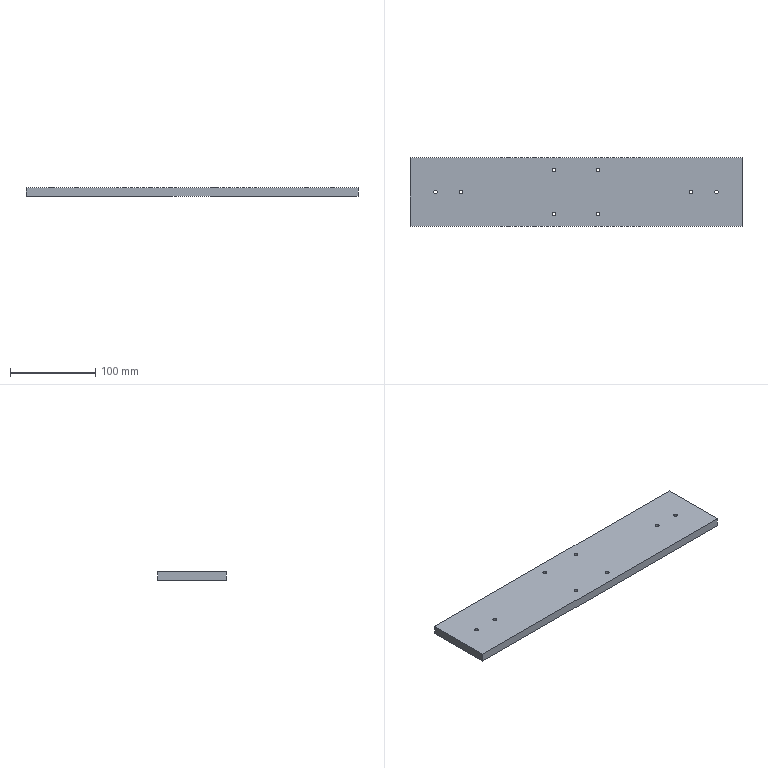Part | STEP file | X77-04402 | 1 solid | 22 faces | box 390 x 80 x 10 mm | volume 310892 mm3 | cylinder 16 | plane 6 | commonest cylinder face diameters 4.2 x16
STEP:
#1=CARTESIAN_POINT('',(162.9,0.,0.));
#2=VERTEX_POINT('',#1);
#3=CARTESIAN_POINT('',(167.1,0.,0.));
#4=VERTEX_POINT('',#3);
#5=CARTESIAN_POINT('',(165.,0.,0.));
#6=DIRECTION('',(0.,0.,1.));
#7=DIRECTION('',(1.,0.,0.));
#8=AXIS2_PLACEMENT_3D('',#5,#6,#7);
#9=CIRCLE('',#8,2.1);
#10=EDGE_CURVE('',#2,#4,#9,.T.);
#11=ORIENTED_EDGE('',*,*,#10,.F.);
#12=CARTESIAN_POINT('',(162.9,0.,10.));
#13=VERTEX_POINT('',#12);
#14=CARTESIAN_POINT('',(162.9,0.,10.));
#15=DIRECTION('',(0.,0.,1.));
#16=VECTOR('',#15,1000.);
#17=LINE('',#14,#16);
#18=EDGE_CURVE('',#2,#13,#17,.T.);
#19=ORIENTED_EDGE('',*,*,#18,.T.);
#20=CARTESIAN_POINT('',(167.1,0.,10.));
#21=VERTEX_POINT('',#20);
#22=CARTESIAN_POINT('',(165.,0.,10.));
#23=DIRECTION('',(0.,0.,1.));
#24=DIRECTION('',(1.,0.,0.));
#25=AXIS2_PLACEMENT_3D('',#22,#23,#24);
#26=CIRCLE('',#25,2.1);
#27=EDGE_CURVE('',#13,#21,#26,.T.);
#28=ORIENTED_EDGE('',*,*,#27,.T.);
#29=CARTESIAN_POINT('',(167.1,0.,10.));
#30=DIRECTION('',(0.,0.,1.));
#31=VECTOR('',#30,1000.);
#32=LINE('',#29,#31);
#33=EDGE_CURVE('',#4,#21,#32,.T.);
#34=ORIENTED_EDGE('',*,*,#33,.F.);
#35=EDGE_LOOP('',(#11,#19,#28,#34));
#36=FACE_OUTER_BOUND('',#35,.T.);
#37=CARTESIAN_POINT('',(165.,0.,10.));
#38=DIRECTION('',(0.,0.,1.));
#39=DIRECTION('',(1.,0.,0.));
#40=AXIS2_PLACEMENT_3D('',#37,#38,#39);
#41=CYLINDRICAL_SURFACE('',#40,2.1);
#42=ADVANCED_FACE('',(#36),#41,.F.);
#43=CARTESIAN_POINT('',(132.9,0.,0.));
#44=VERTEX_POINT('',#43);
#45=CARTESIAN_POINT('',(137.1,0.,0.));
#46=VERTEX_POINT('',#45);
#47=CARTESIAN_POINT('',(135.,0.,0.));
#48=DIRECTION('',(0.,0.,1.));
#49=DIRECTION('',(1.,0.,0.));
#50=AXIS2_PLACEMENT_3D('',#47,#48,#49);
#51=CIRCLE('',#50,2.1);
#52=EDGE_CURVE('',#44,#46,#51,.T.);
#53=ORIENTED_EDGE('',*,*,#52,.F.);
#54=CARTESIAN_POINT('',(132.9,0.,10.));
#55=VERTEX_POINT('',#54);
#56=CARTESIAN_POINT('',(132.9,0.,10.));
#57=DIRECTION('',(0.,0.,1.));
#58=VECTOR('',#57,1000.);
#59=LINE('',#56,#58);
#60=EDGE_CURVE('',#44,#55,#59,.T.);
#61=ORIENTED_EDGE('',*,*,#60,.T.);
#62=CARTESIAN_POINT('',(137.1,0.,10.));
#63=VERTEX_POINT('',#62);
#64=CARTESIAN_POINT('',(135.,0.,10.));
#65=DIRECTION('',(0.,0.,1.));
#66=DIRECTION('',(1.,0.,0.));
#67=AXIS2_PLACEMENT_3D('',#64,#65,#66);
#68=CIRCLE('',#67,2.1);
#69=EDGE_CURVE('',#55,#63,#68,.T.);
#70=ORIENTED_EDGE('',*,*,#69,.T.);
#71=CARTESIAN_POINT('',(137.1,0.,10.));
#72=DIRECTION('',(0.,0.,1.));
#73=VECTOR('',#72,1000.);
#74=LINE('',#71,#73);
#75=EDGE_CURVE('',#46,#63,#74,.T.);
#76=ORIENTED_EDGE('',*,*,#75,.F.);
#77=EDGE_LOOP('',(#53,#61,#70,#76));
#78=FACE_OUTER_BOUND('',#77,.T.);
#79=CARTESIAN_POINT('',(135.,0.,10.));
#80=DIRECTION('',(0.,0.,1.));
#81=DIRECTION('',(1.,0.,0.));
#82=AXIS2_PLACEMENT_3D('',#79,#80,#81);
#83=CYLINDRICAL_SURFACE('',#82,2.1);
#84=ADVANCED_FACE('',(#78),#83,.F.);
#85=CARTESIAN_POINT('',(-137.1,0.,0.));
#86=VERTEX_POINT('',#85);
#87=CARTESIAN_POINT('',(-132.9,0.,0.));
#88=VERTEX_POINT('',#87);
#89=CARTESIAN_POINT('',(-135.,0.,0.));
#90=DIRECTION('',(0.,0.,1.));
#91=DIRECTION('',(1.,0.,0.));
#92=AXIS2_PLACEMENT_3D('',#89,#90,#91);
#93=CIRCLE('',#92,2.1);
#94=EDGE_CURVE('',#86,#88,#93,.T.);
#95=ORIENTED_EDGE('',*,*,#94,.F.);
#96=CARTESIAN_POINT('',(-137.1,0.,10.));
#97=VERTEX_POINT('',#96);
#98=CARTESIAN_POINT('',(-137.1,0.,10.));
#99=DIRECTION('',(0.,0.,1.));
#100=VECTOR('',#99,1000.);
#101=LINE('',#98,#100);
#102=EDGE_CURVE('',#86,#97,#101,.T.);
#103=ORIENTED_EDGE('',*,*,#102,.T.);
#104=CARTESIAN_POINT('',(-132.9,0.,10.));
#105=VERTEX_POINT('',#104);
#106=CARTESIAN_POINT('',(-135.,0.,10.));
#107=DIRECTION('',(0.,0.,1.));
#108=DIRECTION('',(1.,0.,0.));
#109=AXIS2_PLACEMENT_3D('',#106,#107,#108);
#110=CIRCLE('',#109,2.1);
#111=EDGE_CURVE('',#97,#105,#110,.T.);
#112=ORIENTED_EDGE('',*,*,#111,.T.);
#113=CARTESIAN_POINT('',(-132.9,0.,10.));
#114=DIRECTION('',(0.,0.,1.));
#115=VECTOR('',#114,1000.);
#116=LINE('',#113,#115);
#117=EDGE_CURVE('',#88,#105,#116,.T.);
#118=ORIENTED_EDGE('',*,*,#117,.F.);
#119=EDGE_LOOP('',(#95,#103,#112,#118));
#120=FACE_OUTER_BOUND('',#119,.T.);
#121=CARTESIAN_POINT('',(-135.,0.,10.));
#122=DIRECTION('',(0.,0.,1.));
#123=DIRECTION('',(1.,0.,0.));
#124=AXIS2_PLACEMENT_3D('',#121,#122,#123);
#125=CYLINDRICAL_SURFACE('',#124,2.1);
#126=ADVANCED_FACE('',(#120),#125,.F.);
#127=CARTESIAN_POINT('',(-167.1,0.,0.));
#128=VERTEX_POINT('',#127);
#129=CARTESIAN_POINT('',(-162.9,0.,0.));
#130=VERTEX_POINT('',#129);
#131=CARTESIAN_POINT('',(-165.,0.,0.));
#132=DIRECTION('',(0.,0.,1.));
#133=DIRECTION('',(1.,0.,0.));
#134=AXIS2_PLACEMENT_3D('',#131,#132,#133);
#135=CIRCLE('',#134,2.1);
#136=EDGE_CURVE('',#128,#130,#135,.T.);
#137=ORIENTED_EDGE('',*,*,#136,.F.);
#138=CARTESIAN_POINT('',(-167.1,0.,10.));
#139=VERTEX_POINT('',#138);
#140=CARTESIAN_POINT('',(-167.1,0.,10.));
#141=DIRECTION('',(0.,0.,1.));
#142=VECTOR('',#141,1000.);
#143=LINE('',#140,#142);
#144=EDGE_CURVE('',#128,#139,#143,.T.);
#145=ORIENTED_EDGE('',*,*,#144,.T.);
#146=CARTESIAN_POINT('',(-162.9,0.,10.));
#147=VERTEX_POINT('',#146);
#148=CARTESIAN_POINT('',(-165.,0.,10.));
#149=DIRECTION('',(0.,0.,1.));
#150=DIRECTION('',(1.,0.,0.));
#151=AXIS2_PLACEMENT_3D('',#148,#149,#150);
#152=CIRCLE('',#151,2.1);
#153=EDGE_CURVE('',#139,#147,#152,.T.);
#154=ORIENTED_EDGE('',*,*,#153,.T.);
#155=CARTESIAN_POINT('',(-162.9,0.,10.));
#156=DIRECTION('',(0.,0.,1.));
#157=VECTOR('',#156,1000.);
#158=LINE('',#155,#157);
#159=EDGE_CURVE('',#130,#147,#158,.T.);
#160=ORIENTED_EDGE('',*,*,#159,.F.);
#161=EDGE_LOOP('',(#137,#145,#154,#160));
#162=FACE_OUTER_BOUND('',#161,.T.);
#163=CARTESIAN_POINT('',(-165.,0.,10.));
#164=DIRECTION('',(0.,0.,1.));
#165=DIRECTION('',(1.,0.,0.));
#166=AXIS2_PLACEMENT_3D('',#163,#164,#165);
#167=CYLINDRICAL_SURFACE('',#166,2.1);
#168=ADVANCED_FACE('',(#162),#167,.F.);
#169=CARTESIAN_POINT('',(-28.1,26.,10.));
#170=VERTEX_POINT('',#169);
#171=CARTESIAN_POINT('',(-23.9,26.,10.));
#172=VERTEX_POINT('',#171);
#173=CARTESIAN_POINT('',(-26.,26.,10.));
#174=DIRECTION('',(0.,0.,1.));
#175=DIRECTION('',(1.,0.,0.));
#176=AXIS2_PLACEMENT_3D('',#173,#174,#175);
#177=CIRCLE('',#176,2.1);
#178=EDGE_CURVE('',#170,#172,#177,.T.);
#179=ORIENTED_EDGE('',*,*,#178,.T.);
#180=CARTESIAN_POINT('',(-23.9,26.,0.));
#181=VERTEX_POINT('',#180);
#182=CARTESIAN_POINT('',(-23.9,26.,0.));
#183=DIRECTION('',(0.,0.,-1.));
#184=VECTOR('',#183,1000.);
#185=LINE('',#182,#184);
#186=EDGE_CURVE('',#172,#181,#185,.T.);
#187=ORIENTED_EDGE('',*,*,#186,.T.);
#188=CARTESIAN_POINT('',(-28.1,26.,0.));
#189=VERTEX_POINT('',#188);
#190=CARTESIAN_POINT('',(-26.,26.,0.));
#191=DIRECTION('',(0.,0.,-1.));
#192=DIRECTION('',(-1.,0.,0.));
#193=AXIS2_PLACEMENT_3D('',#190,#191,#192);
#194=CIRCLE('',#193,2.1);
#195=EDGE_CURVE('',#181,#189,#194,.T.);
#196=ORIENTED_EDGE('',*,*,#195,.T.);
#197=CARTESIAN_POINT('',(-28.1,26.,0.));
#198=DIRECTION('',(0.,0.,-1.));
#199=VECTOR('',#198,1000.);
#200=LINE('',#197,#199);
#201=EDGE_CURVE('',#170,#189,#200,.T.);
#202=ORIENTED_EDGE('',*,*,#201,.F.);
#203=EDGE_LOOP('',(#179,#187,#196,#202));
#204=FACE_OUTER_BOUND('',#203,.T.);
#205=CARTESIAN_POINT('',(-26.,26.,0.));
#206=DIRECTION('',(0.,0.,-1.));
#207=DIRECTION('',(-1.,0.,0.));
#208=AXIS2_PLACEMENT_3D('',#205,#206,#207);
#209=CYLINDRICAL_SURFACE('',#208,2.1);
#210=ADVANCED_FACE('',(#204),#209,.F.);
#211=CARTESIAN_POINT('',(23.9,26.,10.));
#212=VERTEX_POINT('',#211);
#213=CARTESIAN_POINT('',(28.1,26.,10.));
#214=VERTEX_POINT('',#213);
#215=CARTESIAN_POINT('',(26.,26.,10.));
#216=DIRECTION('',(0.,0.,1.));
#217=DIRECTION('',(1.,0.,0.));
#218=AXIS2_PLACEMENT_3D('',#215,#216,#217);
#219=CIRCLE('',#218,2.1);
#220=EDGE_CURVE('',#212,#214,#219,.T.);
#221=ORIENTED_EDGE('',*,*,#220,.T.);
#222=CARTESIAN_POINT('',(28.1,26.,0.));
#223=VERTEX_POINT('',#222);
#224=CARTESIAN_POINT('',(28.1,26.,0.));
#225=DIRECTION('',(0.,0.,-1.));
#226=VECTOR('',#225,1000.);
#227=LINE('',#224,#226);
#228=EDGE_CURVE('',#214,#223,#227,.T.);
#229=ORIENTED_EDGE('',*,*,#228,.T.);
#230=CARTESIAN_POINT('',(23.9,26.,0.));
#231=VERTEX_POINT('',#230);
#232=CARTESIAN_POINT('',(26.,26.,0.));
#233=DIRECTION('',(0.,0.,-1.));
#234=DIRECTION('',(-1.,0.,0.));
#235=AXIS2_PLACEMENT_3D('',#232,#233,#234);
#236=CIRCLE('',#235,2.1);
#237=EDGE_CURVE('',#223,#231,#236,.T.);
#238=ORIENTED_EDGE('',*,*,#237,.T.);
#239=CARTESIAN_POINT('',(23.9,26.,0.));
#240=DIRECTION('',(0.,0.,-1.));
#241=VECTOR('',#240,1000.);
#242=LINE('',#239,#241);
#243=EDGE_CURVE('',#212,#231,#242,.T.);
#244=ORIENTED_EDGE('',*,*,#243,.F.);
#245=EDGE_LOOP('',(#221,#229,#238,#244));
#246=FACE_OUTER_BOUND('',#245,.T.);
#247=CARTESIAN_POINT('',(26.,26.,0.));
#248=DIRECTION('',(0.,0.,-1.));
#249=DIRECTION('',(-1.,0.,0.));
#250=AXIS2_PLACEMENT_3D('',#247,#248,#249);
#251=CYLINDRICAL_SURFACE('',#250,2.1);
#252=ADVANCED_FACE('',(#246),#251,.F.);
#253=CARTESIAN_POINT('',(-28.1,-26.,10.));
#254=VERTEX_POINT('',#253);
#255=CARTESIAN_POINT('',(-23.9,-26.,10.));
#256=VERTEX_POINT('',#255);
#257=CARTESIAN_POINT('',(-26.,-26.,10.));
#258=DIRECTION('',(0.,0.,1.));
#259=DIRECTION('',(1.,0.,0.));
#260=AXIS2_PLACEMENT_3D('',#257,#258,#259);
#261=CIRCLE('',#260,2.1);
#262=EDGE_CURVE('',#254,#256,#261,.T.);
#263=ORIENTED_EDGE('',*,*,#262,.T.);
#264=CARTESIAN_POINT('',(-23.9,-26.,0.));
#265=VERTEX_POINT('',#264);
#266=CARTESIAN_POINT('',(-23.9,-26.,0.));
#267=DIRECTION('',(0.,0.,-1.));
#268=VECTOR('',#267,1000.);
#269=LINE('',#266,#268);
#270=EDGE_CURVE('',#256,#265,#269,.T.);
#271=ORIENTED_EDGE('',*,*,#270,.T.);
#272=CARTESIAN_POINT('',(-28.1,-26.,0.));
#273=VERTEX_POINT('',#272);
#274=CARTESIAN_POINT('',(-26.,-26.,0.));
#275=DIRECTION('',(0.,0.,-1.));
#276=DIRECTION('',(-1.,0.,0.));
#277=AXIS2_PLACEMENT_3D('',#274,#275,#276);
#278=CIRCLE('',#277,2.1);
#279=EDGE_CURVE('',#265,#273,#278,.T.);
#280=ORIENTED_EDGE('',*,*,#279,.T.);
#281=CARTESIAN_POINT('',(-28.1,-26.,0.));
#282=DIRECTION('',(0.,0.,-1.));
#283=VECTOR('',#282,1000.);
#284=LINE('',#281,#283);
#285=EDGE_CURVE('',#254,#273,#284,.T.);
#286=ORIENTED_EDGE('',*,*,#285,.F.);
#287=EDGE_LOOP('',(#263,#271,#280,#286));
#288=FACE_OUTER_BOUND('',#287,.T.);
#289=CARTESIAN_POINT('',(-26.,-26.,0.));
#290=DIRECTION('',(0.,0.,-1.));
#291=DIRECTION('',(-1.,0.,0.));
#292=AXIS2_PLACEMENT_3D('',#289,#290,#291);
#293=CYLINDRICAL_SURFACE('',#292,2.1);
#294=ADVANCED_FACE('',(#288),#293,.F.);
#295=CARTESIAN_POINT('',(23.9,-26.,10.));
#296=VERTEX_POINT('',#295);
#297=CARTESIAN_POINT('',(28.1,-26.,10.));
#298=VERTEX_POINT('',#297);
#299=CARTESIAN_POINT('',(26.,-26.,10.));
#300=DIRECTION('',(0.,0.,1.));
#301=DIRECTION('',(1.,0.,0.));
#302=AXIS2_PLACEMENT_3D('',#299,#300,#301);
#303=CIRCLE('',#302,2.1);
#304=EDGE_CURVE('',#296,#298,#303,.T.);
#305=ORIENTED_EDGE('',*,*,#304,.T.);
#306=CARTESIAN_POINT('',(28.1,-26.,0.));
#307=VERTEX_POINT('',#306);
#308=CARTESIAN_POINT('',(28.1,-26.,0.));
#309=DIRECTION('',(0.,0.,-1.));
#310=VECTOR('',#309,1000.);
#311=LINE('',#308,#310);
#312=EDGE_CURVE('',#298,#307,#311,.T.);
#313=ORIENTED_EDGE('',*,*,#312,.T.);
#314=CARTESIAN_POINT('',(23.9,-26.,0.));
#315=VERTEX_POINT('',#314);
#316=CARTESIAN_POINT('',(26.,-26.,0.));
#317=DIRECTION('',(0.,0.,-1.));
#318=DIRECTION('',(-1.,0.,0.));
#319=AXIS2_PLACEMENT_3D('',#316,#317,#318);
#320=CIRCLE('',#319,2.1);
#321=EDGE_CURVE('',#307,#315,#320,.T.);
#322=ORIENTED_EDGE('',*,*,#321,.T.);
#323=CARTESIAN_POINT('',(23.9,-26.,0.));
#324=DIRECTION('',(0.,0.,-1.));
#325=VECTOR('',#324,1000.);
#326=LINE('',#323,#325);
#327=EDGE_CURVE('',#296,#315,#326,.T.);
#328=ORIENTED_EDGE('',*,*,#327,.F.);
#329=EDGE_LOOP('',(#305,#313,#322,#328));
#330=FACE_OUTER_BOUND('',#329,.T.);
#331=CARTESIAN_POINT('',(26.,-26.,0.));
#332=DIRECTION('',(0.,0.,-1.));
#333=DIRECTION('',(-1.,0.,0.));
#334=AXIS2_PLACEMENT_3D('',#331,#332,#333);
#335=CYLINDRICAL_SURFACE('',#334,2.1);
#336=ADVANCED_FACE('',(#330),#335,.F.);
#337=CARTESIAN_POINT('',(195.,-40.,0.));
#338=VERTEX_POINT('',#337);
#339=CARTESIAN_POINT('',(195.,40.,0.));
#340=VERTEX_POINT('',#339);
#341=CARTESIAN_POINT('',(195.,40.,0.));
#342=DIRECTION('',(0.,1.,0.));
#343=VECTOR('',#342,1000.);
#344=LINE('',#341,#343);
#345=EDGE_CURVE('',#338,#340,#344,.T.);
#346=ORIENTED_EDGE('',*,*,#345,.T.);
#347=CARTESIAN_POINT('',(195.,40.,10.));
#348=VERTEX_POINT('',#347);
#349=CARTESIAN_POINT('',(195.,40.,10.));
#350=DIRECTION('',(0.,0.,-1.));
#351=VECTOR('',#350,1000.);
#352=LINE('',#349,#351);
#353=EDGE_CURVE('',#348,#340,#352,.T.);
#354=ORIENTED_EDGE('',*,*,#353,.F.);
#355=CARTESIAN_POINT('',(195.,-40.,10.));
#356=VERTEX_POINT('',#355);
#357=CARTESIAN_POINT('',(195.,40.,10.));
#358=DIRECTION('',(0.,1.,0.));
#359=VECTOR('',#358,1000.);
#360=LINE('',#357,#359);
#361=EDGE_CURVE('',#356,#348,#360,.T.);
#362=ORIENTED_EDGE('',*,*,#361,.F.);
#363=CARTESIAN_POINT('',(195.,-40.,10.));
#364=DIRECTION('',(0.,0.,-1.));
#365=VECTOR('',#364,1000.);
#366=LINE('',#363,#365);
#367=EDGE_CURVE('',#356,#338,#366,.T.);
#368=ORIENTED_EDGE('',*,*,#367,.T.);
#369=EDGE_LOOP('',(#346,#354,#362,#368));
#370=FACE_OUTER_BOUND('',#369,.T.);
#371=CARTESIAN_POINT('',(195.,40.,10.));
#372=DIRECTION('',(-1.,0.,0.));
#373=DIRECTION('',(0.,-1.,0.));
#374=AXIS2_PLACEMENT_3D('',#371,#372,#373);
#375=PLANE('',#374);
#376=ADVANCED_FACE('',(#370),#375,.F.);
#377=CARTESIAN_POINT('',(-195.,40.,0.));
#378=VERTEX_POINT('',#377);
#379=CARTESIAN_POINT('',(-195.,40.,0.));
#380=DIRECTION('',(-1.,0.,0.));
#381=VECTOR('',#380,1000.);
#382=LINE('',#379,#381);
#383=EDGE_CURVE('',#340,#378,#382,.T.);
#384=ORIENTED_EDGE('',*,*,#383,.T.);
#385=CARTESIAN_POINT('',(-195.,40.,10.));
#386=VERTEX_POINT('',#385);
#387=CARTESIAN_POINT('',(-195.,40.,10.));
#388=DIRECTION('',(0.,0.,-1.));
#389=VECTOR('',#388,1000.);
#390=LINE('',#387,#389);
#391=EDGE_CURVE('',#386,#378,#390,.T.);
#392=ORIENTED_EDGE('',*,*,#391,.F.);
#393=CARTESIAN_POINT('',(-195.,40.,10.));
#394=DIRECTION('',(-1.,0.,0.));
#395=VECTOR('',#394,1000.);
#396=LINE('',#393,#395);
#397=EDGE_CURVE('',#348,#386,#396,.T.);
#398=ORIENTED_EDGE('',*,*,#397,.F.);
#399=ORIENTED_EDGE('',*,*,#353,.T.);
#400=EDGE_LOOP('',(#384,#392,#398,#399));
#401=FACE_OUTER_BOUND('',#400,.T.);
#402=CARTESIAN_POINT('',(-195.,40.,10.));
#403=DIRECTION('',(0.,-1.,0.));
#404=DIRECTION('',(0.,0.,-1.));
#405=AXIS2_PLACEMENT_3D('',#402,#403,#404);
#406=PLANE('',#405);
#407=ADVANCED_FACE('',(#401),#406,.F.);
#408=CARTESIAN_POINT('',(-195.,-40.,0.));
#409=VERTEX_POINT('',#408);
#410=CARTESIAN_POINT('',(-195.,40.,0.));
#411=DIRECTION('',(0.,-1.,0.));
#412=VECTOR('',#411,1000.);
#413=LINE('',#410,#412);
#414=EDGE_CURVE('',#378,#409,#413,.T.);
#415=ORIENTED_EDGE('',*,*,#414,.T.);
#416=CARTESIAN_POINT('',(-195.,-40.,10.));
#417=VERTEX_POINT('',#416);
#418=CARTESIAN_POINT('',(-195.,-40.,10.));
#419=DIRECTION('',(0.,0.,-1.));
#420=VECTOR('',#419,1000.);
#421=LINE('',#418,#420);
#422=EDGE_CURVE('',#417,#409,#421,.T.);
#423=ORIENTED_EDGE('',*,*,#422,.F.);
#424=CARTESIAN_POINT('',(-195.,40.,10.));
#425=DIRECTION('',(0.,-1.,0.));
#426=VECTOR('',#425,1000.);
#427=LINE('',#424,#426);
#428=EDGE_CURVE('',#386,#417,#427,.T.);
#429=ORIENTED_EDGE('',*,*,#428,.F.);
#430=ORIENTED_EDGE('',*,*,#391,.T.);
#431=EDGE_LOOP('',(#415,#423,#429,#430));
#432=FACE_OUTER_BOUND('',#431,.T.);
#433=CARTESIAN_POINT('',(-195.,40.,10.));
#434=DIRECTION('',(1.,0.,0.));
#435=DIRECTION('',(0.,0.,-1.));
#436=AXIS2_PLACEMENT_3D('',#433,#434,#435);
#437=PLANE('',#436);
#438=ADVANCED_FACE('',(#432),#437,.F.);
#439=CARTESIAN_POINT('',(-195.,-40.,0.));
#440=DIRECTION('',(1.,0.,0.));
#441=VECTOR('',#440,1000.);
#442=LINE('',#439,#441);
#443=EDGE_CURVE('',#409,#338,#442,.T.);
#444=ORIENTED_EDGE('',*,*,#443,.T.);
#445=ORIENTED_EDGE('',*,*,#367,.F.);
#446=CARTESIAN_POINT('',(-195.,-40.,10.));
#447=DIRECTION('',(1.,0.,0.));
#448=VECTOR('',#447,1000.);
#449=LINE('',#446,#448);
#450=EDGE_CURVE('',#417,#356,#449,.T.);
#451=ORIENTED_EDGE('',*,*,#450,.F.);
#452=ORIENTED_EDGE('',*,*,#422,.T.);
#453=EDGE_LOOP('',(#444,#445,#451,#452));
#454=FACE_OUTER_BOUND('',#453,.T.);
#455=CARTESIAN_POINT('',(-195.,-40.,10.));
#456=DIRECTION('',(0.,1.,0.));
#457=DIRECTION('',(0.,0.,1.));
#458=AXIS2_PLACEMENT_3D('',#455,#456,#457);
#459=PLANE('',#458);
#460=ADVANCED_FACE('',(#454),#459,.F.);
#461=CARTESIAN_POINT('',(165.,0.,10.));
#462=DIRECTION('',(0.,0.,1.));
#463=DIRECTION('',(1.,0.,0.));
#464=AXIS2_PLACEMENT_3D('',#461,#462,#463);
#465=CIRCLE('',#464,2.1);
#466=EDGE_CURVE('',#21,#13,#465,.T.);
#467=ORIENTED_EDGE('',*,*,#466,.F.);
#468=ORIENTED_EDGE('',*,*,#27,.F.);
#469=EDGE_LOOP('',(#467,#468));
#470=FACE_BOUND('',#469,.T.);
#471=CARTESIAN_POINT('',(135.,0.,10.));
#472=DIRECTION('',(0.,0.,1.));
#473=DIRECTION('',(1.,0.,0.));
#474=AXIS2_PLACEMENT_3D('',#471,#472,#473);
#475=CIRCLE('',#474,2.1);
#476=EDGE_CURVE('',#63,#55,#475,.T.);
#477=ORIENTED_EDGE('',*,*,#476,.F.);
#478=ORIENTED_EDGE('',*,*,#69,.F.);
#479=EDGE_LOOP('',(#477,#478));
#480=FACE_BOUND('',#479,.T.);
#481=CARTESIAN_POINT('',(-135.,0.,10.));
#482=DIRECTION('',(0.,0.,1.));
#483=DIRECTION('',(1.,0.,0.));
#484=AXIS2_PLACEMENT_3D('',#481,#482,#483);
#485=CIRCLE('',#484,2.1);
#486=EDGE_CURVE('',#105,#97,#485,.T.);
#487=ORIENTED_EDGE('',*,*,#486,.F.);
#488=ORIENTED_EDGE('',*,*,#111,.F.);
#489=EDGE_LOOP('',(#487,#488));
#490=FACE_BOUND('',#489,.T.);
#491=CARTESIAN_POINT('',(-165.,0.,10.));
#492=DIRECTION('',(0.,0.,1.));
#493=DIRECTION('',(1.,0.,0.));
#494=AXIS2_PLACEMENT_3D('',#491,#492,#493);
#495=CIRCLE('',#494,2.1);
#496=EDGE_CURVE('',#147,#139,#495,.T.);
#497=ORIENTED_EDGE('',*,*,#496,.F.);
#498=ORIENTED_EDGE('',*,*,#153,.F.);
#499=EDGE_LOOP('',(#497,#498));
#500=FACE_BOUND('',#499,.T.);
#501=ORIENTED_EDGE('',*,*,#178,.F.);
#502=CARTESIAN_POINT('',(-26.,26.,10.));
#503=DIRECTION('',(0.,0.,1.));
#504=DIRECTION('',(1.,0.,0.));
#505=AXIS2_PLACEMENT_3D('',#502,#503,#504);
#506=CIRCLE('',#505,2.1);
#507=EDGE_CURVE('',#172,#170,#506,.T.);
#508=ORIENTED_EDGE('',*,*,#507,.F.);
#509=EDGE_LOOP('',(#501,#508));
#510=FACE_BOUND('',#509,.T.);
#511=ORIENTED_EDGE('',*,*,#220,.F.);
#512=CARTESIAN_POINT('',(26.,26.,10.));
#513=DIRECTION('',(0.,0.,1.));
#514=DIRECTION('',(1.,0.,0.));
#515=AXIS2_PLACEMENT_3D('',#512,#513,#514);
#516=CIRCLE('',#515,2.1);
#517=EDGE_CURVE('',#214,#212,#516,.T.);
#518=ORIENTED_EDGE('',*,*,#517,.F.);
#519=EDGE_LOOP('',(#511,#518));
#520=FACE_BOUND('',#519,.T.);
#521=ORIENTED_EDGE('',*,*,#262,.F.);
#522=CARTESIAN_POINT('',(-26.,-26.,10.));
#523=DIRECTION('',(0.,0.,1.));
#524=DIRECTION('',(1.,0.,0.));
#525=AXIS2_PLACEMENT_3D('',#522,#523,#524);
#526=CIRCLE('',#525,2.1);
#527=EDGE_CURVE('',#256,#254,#526,.T.);
#528=ORIENTED_EDGE('',*,*,#527,.F.);
#529=EDGE_LOOP('',(#521,#528));
#530=FACE_BOUND('',#529,.T.);
#531=ORIENTED_EDGE('',*,*,#304,.F.);
#532=CARTESIAN_POINT('',(26.,-26.,10.));
#533=DIRECTION('',(0.,0.,1.));
#534=DIRECTION('',(1.,0.,0.));
#535=AXIS2_PLACEMENT_3D('',#532,#533,#534);
#536=CIRCLE('',#535,2.1);
#537=EDGE_CURVE('',#298,#296,#536,.T.);
#538=ORIENTED_EDGE('',*,*,#537,.F.);
#539=EDGE_LOOP('',(#531,#538));
#540=FACE_BOUND('',#539,.T.);
#541=ORIENTED_EDGE('',*,*,#361,.T.);
#542=ORIENTED_EDGE('',*,*,#397,.T.);
#543=ORIENTED_EDGE('',*,*,#428,.T.);
#544=ORIENTED_EDGE('',*,*,#450,.T.);
#545=EDGE_LOOP('',(#541,#542,#543,#544));
#546=FACE_OUTER_BOUND('',#545,.T.);
#547=CARTESIAN_POINT('',(195.,-40.,10.));
#548=DIRECTION('',(0.,0.,1.));
#549=DIRECTION('',(1.,0.,0.));
#550=AXIS2_PLACEMENT_3D('',#547,#548,#549);
#551=PLANE('',#550);
#552=ADVANCED_FACE('',(#470,#480,#490,#500,#510,#520,#530,#540,#546),#551,.T.);
#553=CARTESIAN_POINT('',(165.,0.,0.));
#554=DIRECTION('',(0.,0.,1.));
#555=DIRECTION('',(1.,0.,0.));
#556=AXIS2_PLACEMENT_3D('',#553,#554,#555);
#557=CIRCLE('',#556,2.1);
#558=EDGE_CURVE('',#4,#2,#557,.T.);
#559=ORIENTED_EDGE('',*,*,#558,.T.);
#560=ORIENTED_EDGE('',*,*,#10,.T.);
#561=EDGE_LOOP('',(#559,#560));
#562=FACE_BOUND('',#561,.T.);
#563=CARTESIAN_POINT('',(135.,0.,0.));
#564=DIRECTION('',(0.,0.,1.));
#565=DIRECTION('',(1.,0.,0.));
#566=AXIS2_PLACEMENT_3D('',#563,#564,#565);
#567=CIRCLE('',#566,2.1);
#568=EDGE_CURVE('',#46,#44,#567,.T.);
#569=ORIENTED_EDGE('',*,*,#568,.T.);
#570=ORIENTED_EDGE('',*,*,#52,.T.);
#571=EDGE_LOOP('',(#569,#570));
#572=FACE_BOUND('',#571,.T.);
#573=CARTESIAN_POINT('',(-135.,0.,0.));
#574=DIRECTION('',(0.,0.,1.));
#575=DIRECTION('',(1.,0.,0.));
#576=AXIS2_PLACEMENT_3D('',#573,#574,#575);
#577=CIRCLE('',#576,2.1);
#578=EDGE_CURVE('',#88,#86,#577,.T.);
#579=ORIENTED_EDGE('',*,*,#578,.T.);
#580=ORIENTED_EDGE('',*,*,#94,.T.);
#581=EDGE_LOOP('',(#579,#580));
#582=FACE_BOUND('',#581,.T.);
#583=CARTESIAN_POINT('',(-165.,0.,0.));
#584=DIRECTION('',(0.,0.,1.));
#585=DIRECTION('',(1.,0.,0.));
#586=AXIS2_PLACEMENT_3D('',#583,#584,#585);
#587=CIRCLE('',#586,2.1);
#588=EDGE_CURVE('',#130,#128,#587,.T.);
#589=ORIENTED_EDGE('',*,*,#588,.T.);
#590=ORIENTED_EDGE('',*,*,#136,.T.);
#591=EDGE_LOOP('',(#589,#590));
#592=FACE_BOUND('',#591,.T.);
#593=CARTESIAN_POINT('',(-26.,26.,0.));
#594=DIRECTION('',(0.,0.,-1.));
#595=DIRECTION('',(-1.,0.,0.));
#596=AXIS2_PLACEMENT_3D('',#593,#594,#595);
#597=CIRCLE('',#596,2.1);
#598=EDGE_CURVE('',#189,#181,#597,.T.);
#599=ORIENTED_EDGE('',*,*,#598,.F.);
#600=ORIENTED_EDGE('',*,*,#195,.F.);
#601=EDGE_LOOP('',(#599,#600));
#602=FACE_BOUND('',#601,.T.);
#603=CARTESIAN_POINT('',(26.,26.,0.));
#604=DIRECTION('',(0.,0.,-1.));
#605=DIRECTION('',(-1.,0.,0.));
#606=AXIS2_PLACEMENT_3D('',#603,#604,#605);
#607=CIRCLE('',#606,2.1);
#608=EDGE_CURVE('',#231,#223,#607,.T.);
#609=ORIENTED_EDGE('',*,*,#608,.F.);
#610=ORIENTED_EDGE('',*,*,#237,.F.);
#611=EDGE_LOOP('',(#609,#610));
#612=FACE_BOUND('',#611,.T.);
#613=CARTESIAN_POINT('',(-26.,-26.,0.));
#614=DIRECTION('',(0.,0.,-1.));
#615=DIRECTION('',(-1.,0.,0.));
#616=AXIS2_PLACEMENT_3D('',#613,#614,#615);
#617=CIRCLE('',#616,2.1);
#618=EDGE_CURVE('',#273,#265,#617,.T.);
#619=ORIENTED_EDGE('',*,*,#618,.F.);
#620=ORIENTED_EDGE('',*,*,#279,.F.);
#621=EDGE_LOOP('',(#619,#620));
#622=FACE_BOUND('',#621,.T.);
#623=CARTESIAN_POINT('',(26.,-26.,0.));
#624=DIRECTION('',(0.,0.,-1.));
#625=DIRECTION('',(-1.,0.,0.));
#626=AXIS2_PLACEMENT_3D('',#623,#624,#625);
#627=CIRCLE('',#626,2.1);
#628=EDGE_CURVE('',#315,#307,#627,.T.);
#629=ORIENTED_EDGE('',*,*,#628,.F.);
#630=ORIENTED_EDGE('',*,*,#321,.F.);
#631=EDGE_LOOP('',(#629,#630));
#632=FACE_BOUND('',#631,.T.);
#633=ORIENTED_EDGE('',*,*,#345,.F.);
#634=ORIENTED_EDGE('',*,*,#443,.F.);
#635=ORIENTED_EDGE('',*,*,#414,.F.);
#636=ORIENTED_EDGE('',*,*,#383,.F.);
#637=EDGE_LOOP('',(#633,#634,#635,#636));
#638=FACE_OUTER_BOUND('',#637,.T.);
#639=CARTESIAN_POINT('',(195.,-40.,0.));
#640=DIRECTION('',(0.,0.,1.));
#641=DIRECTION('',(1.,0.,0.));
#642=AXIS2_PLACEMENT_3D('',#639,#640,#641);
#643=PLANE('',#642);
#644=ADVANCED_FACE('',(#562,#572,#582,#592,#602,#612,#622,#632,#638),#643,.F.);
#645=ORIENTED_EDGE('',*,*,#312,.F.);
#646=ORIENTED_EDGE('',*,*,#537,.T.);
#647=ORIENTED_EDGE('',*,*,#327,.T.);
#648=ORIENTED_EDGE('',*,*,#628,.T.);
#649=EDGE_LOOP('',(#645,#646,#647,#648));
#650=FACE_OUTER_BOUND('',#649,.T.);
#651=CARTESIAN_POINT('',(26.,-26.,0.));
#652=DIRECTION('',(0.,0.,-1.));
#653=DIRECTION('',(-1.,0.,0.));
#654=AXIS2_PLACEMENT_3D('',#651,#652,#653);
#655=CYLINDRICAL_SURFACE('',#654,2.1);
#656=ADVANCED_FACE('',(#650),#655,.F.);
#657=ORIENTED_EDGE('',*,*,#270,.F.);
#658=ORIENTED_EDGE('',*,*,#527,.T.);
#659=ORIENTED_EDGE('',*,*,#285,.T.);
#660=ORIENTED_EDGE('',*,*,#618,.T.);
#661=EDGE_LOOP('',(#657,#658,#659,#660));
#662=FACE_OUTER_BOUND('',#661,.T.);
#663=CARTESIAN_POINT('',(-26.,-26.,0.));
#664=DIRECTION('',(0.,0.,-1.));
#665=DIRECTION('',(-1.,0.,0.));
#666=AXIS2_PLACEMENT_3D('',#663,#664,#665);
#667=CYLINDRICAL_SURFACE('',#666,2.1);
#668=ADVANCED_FACE('',(#662),#667,.F.);
#669=ORIENTED_EDGE('',*,*,#228,.F.);
#670=ORIENTED_EDGE('',*,*,#517,.T.);
#671=ORIENTED_EDGE('',*,*,#243,.T.);
#672=ORIENTED_EDGE('',*,*,#608,.T.);
#673=EDGE_LOOP('',(#669,#670,#671,#672));
#674=FACE_OUTER_BOUND('',#673,.T.);
#675=CARTESIAN_POINT('',(26.,26.,0.));
#676=DIRECTION('',(0.,0.,-1.));
#677=DIRECTION('',(-1.,0.,0.));
#678=AXIS2_PLACEMENT_3D('',#675,#676,#677);
#679=CYLINDRICAL_SURFACE('',#678,2.1);
#680=ADVANCED_FACE('',(#674),#679,.F.);
#681=ORIENTED_EDGE('',*,*,#186,.F.);
#682=ORIENTED_EDGE('',*,*,#507,.T.);
#683=ORIENTED_EDGE('',*,*,#201,.T.);
#684=ORIENTED_EDGE('',*,*,#598,.T.);
#685=EDGE_LOOP('',(#681,#682,#683,#684));
#686=FACE_OUTER_BOUND('',#685,.T.);
#687=CARTESIAN_POINT('',(-26.,26.,0.));
#688=DIRECTION('',(0.,0.,-1.));
#689=DIRECTION('',(-1.,0.,0.));
#690=AXIS2_PLACEMENT_3D('',#687,#688,#689);
#691=CYLINDRICAL_SURFACE('',#690,2.1);
#692=ADVANCED_FACE('',(#686),#691,.F.);
#693=ORIENTED_EDGE('',*,*,#144,.F.);
#694=ORIENTED_EDGE('',*,*,#588,.F.);
#695=ORIENTED_EDGE('',*,*,#159,.T.);
#696=ORIENTED_EDGE('',*,*,#496,.T.);
#697=EDGE_LOOP('',(#693,#694,#695,#696));
#698=FACE_OUTER_BOUND('',#697,.T.);
#699=CARTESIAN_POINT('',(-165.,0.,10.));
#700=DIRECTION('',(0.,0.,1.));
#701=DIRECTION('',(1.,0.,0.));
#702=AXIS2_PLACEMENT_3D('',#699,#700,#701);
#703=CYLINDRICAL_SURFACE('',#702,2.1);
#704=ADVANCED_FACE('',(#698),#703,.F.);
#705=ORIENTED_EDGE('',*,*,#102,.F.);
#706=ORIENTED_EDGE('',*,*,#578,.F.);
#707=ORIENTED_EDGE('',*,*,#117,.T.);
#708=ORIENTED_EDGE('',*,*,#486,.T.);
#709=EDGE_LOOP('',(#705,#706,#707,#708));
#710=FACE_OUTER_BOUND('',#709,.T.);
#711=CARTESIAN_POINT('',(-135.,0.,10.));
#712=DIRECTION('',(0.,0.,1.));
#713=DIRECTION('',(1.,0.,0.));
#714=AXIS2_PLACEMENT_3D('',#711,#712,#713);
#715=CYLINDRICAL_SURFACE('',#714,2.1);
#716=ADVANCED_FACE('',(#710),#715,.F.);
#717=ORIENTED_EDGE('',*,*,#60,.F.);
#718=ORIENTED_EDGE('',*,*,#568,.F.);
#719=ORIENTED_EDGE('',*,*,#75,.T.);
#720=ORIENTED_EDGE('',*,*,#476,.T.);
#721=EDGE_LOOP('',(#717,#718,#719,#720));
#722=FACE_OUTER_BOUND('',#721,.T.);
#723=CARTESIAN_POINT('',(135.,0.,10.));
#724=DIRECTION('',(0.,0.,1.));
#725=DIRECTION('',(1.,0.,0.));
#726=AXIS2_PLACEMENT_3D('',#723,#724,#725);
#727=CYLINDRICAL_SURFACE('',#726,2.1);
#728=ADVANCED_FACE('',(#722),#727,.F.);
#729=ORIENTED_EDGE('',*,*,#18,.F.);
#730=ORIENTED_EDGE('',*,*,#558,.F.);
#731=ORIENTED_EDGE('',*,*,#33,.T.);
#732=ORIENTED_EDGE('',*,*,#466,.T.);
#733=EDGE_LOOP('',(#729,#730,#731,#732));
#734=FACE_OUTER_BOUND('',#733,.T.);
#735=CARTESIAN_POINT('',(165.,0.,10.));
#736=DIRECTION('',(0.,0.,1.));
#737=DIRECTION('',(1.,0.,0.));
#738=AXIS2_PLACEMENT_3D('',#735,#736,#737);
#739=CYLINDRICAL_SURFACE('',#738,2.1);
#740=ADVANCED_FACE('',(#734),#739,.F.);
#741=CLOSED_SHELL('',(#42,#84,#126,#168,#210,#252,#294,#336,#376,#407,#438,#460,#552,#644,#656,#668,#680,#692,#704,#716,#728,#740));
#742=MANIFOLD_SOLID_BREP('',#741);
#743=CARTESIAN_POINT('',(0.,0.,0.));
#744=DIRECTION('',(0.,0.,1.));
#745=DIRECTION('',(1.,0.,0.));
#746=AXIS2_PLACEMENT_3D('',#743,#744,#745);
#747=(LENGTH_UNIT()NAMED_UNIT(*)SI_UNIT(.MILLI.,.METRE.));
#748=UNCERTAINTY_MEASURE_WITH_UNIT(LENGTH_MEASURE(0.00001),#747,'','');
#749=(NAMED_UNIT(*)PLANE_ANGLE_UNIT()SI_UNIT($,.RADIAN.));
#750=(NAMED_UNIT(*)SI_UNIT($,.STERADIAN.)SOLID_ANGLE_UNIT());
#751=(GEOMETRIC_REPRESENTATION_CONTEXT(3)GLOBAL_UNCERTAINTY_ASSIGNED_CONTEXT((#748))GLOBAL_UNIT_ASSIGNED_CONTEXT((#747,#749,#750))REPRESENTATION_CONTEXT('',''));
#752=ADVANCED_BREP_SHAPE_REPRESENTATION('',(#742,#746),#751);